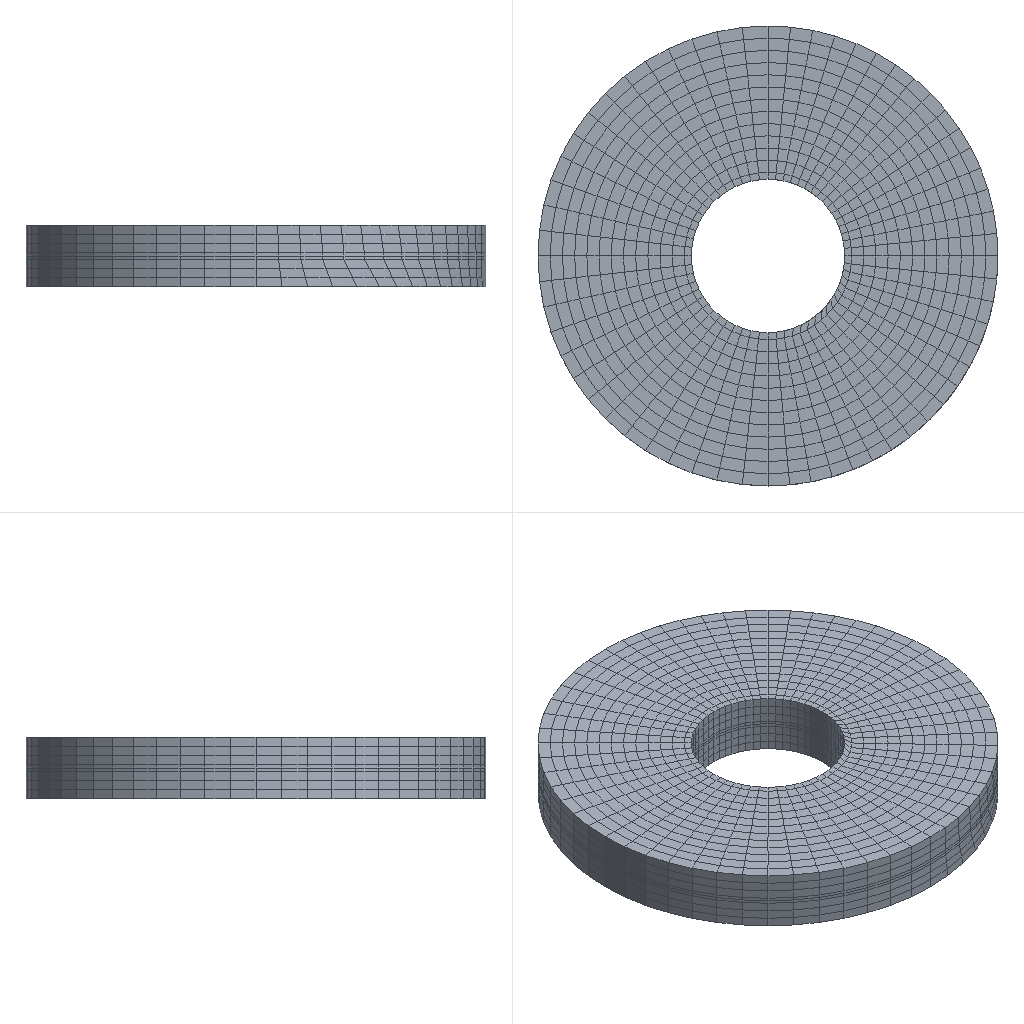Simulation study | abaqus
Set-up summary:
category,name,step,type,value,unit,region
solver,abaqus
solver,version,,,Abaqus/Explicit 2020
units,not stated in the deck,,not stated
analysis,deck,,transient,transient
load_step,Step-1,Step-1,transient
load_step,requested,,,1
mesh,nodes,,,8840
mesh,elements,,,7524
element_type,C3D8,,solid,6240
element_type,R3D3,,rigid,14
element_type,R3D4,,rigid,1270
load,load commands in deck,,count,1
bc,support commands in deck,,count,1
material,MATERIAL-1,,in results
material,MATERIAL-1-COPY,,in results
check,setup vs results,,match,"per instance, exact: element labels, types and connectivity; labels of the nodes the elements use; coordinates not compared"
Abaqus input file, long lists of numbers shortened:
*Heading
** Job name: Job-3 Model name: Model-1-Copy-Copy
** Generated by: Abaqus/CAE 2020
*Preprint, echo=NO, model=NO, history=NO, contact=NO
**
** PARTS
**
*Part, name=Part-1
*Node
      1,   1.118,  -2.236,           4.
      2,   1.118,  -2.236,           0.
** (1277 more lines like these left out)
*Element, type=R3D4
  1,   1,   3, 105, 156
  2,   3,   4, 106, 105
** (1268 more lines like these left out)
*Element, type=R3D3
677,  963,  757,  736
678,  987,  863,  818
** (12 more lines like these left out)
*Node
   1280,           0., -1.5308085e-16,           4.
*Nset, nset=Part-1-RefPt_, internal
1280,
*Elset, elset=Part-1, generate
    1,  1284,     1
*End Part
**
*Part, name=Part-2
*Node
      1,           0.,   2.723,  0.9
      2,           0.,          7.5,  0.9
** (7558 more lines like these left out)
*Element, type=C3D8
  1,    5,  117, 1334,  168,    1,   65, 1169,  116
  2,  117,  118, 1335, 1334,   65,   66, 1170, 1169
** (6238 more lines like these left out)
*Nset, nset=Set-3, generate
    1,  7560,     1
*Elset, elset=Set-3, generate
    1,  6240,     1
*Nset, nset=Set-11
    1,    2,    3,    4,    5,    6,    7,    8,    9,   10,   11,   12,   13,   14,   15,   16
   25,   26,   27,   28,   29,   30,   31,   32,   33,   39,   40,   41,   42,   43,   44,   47
** (437 more lines like these left out)
*Elset, elset=Set-11
    1,    2,    3,    4,    5,    6,    7,    8,    9,   10,   11,   12,   13,   14,   15,   16
   17,   18,   19,   20,   21,   22,   23,   24,   25,   26,   27,   28,   29,   30,   31,   32
** (358 more lines like these left out)
*Nset, nset=Set-12, generate
    1,  7560,     1
*Elset, elset=Set-12, generate
    1,  6240,     1
*Nset, nset=Set-9
    1,    2,    3,    4,    5,    6,    7,    8,    9,   10,   11,   12,   13,   14,   15,   16
   17,   18,   21,   22,   25,   26,   27,   28,   29,   30,   31,   32,   33,   34,   35,   36
** (467 more lines like these left out)
*Elset, elset=Set-9
    1,    2,    3,    4,    5,    6,    7,    8,    9,   10,   11,   12,   13,   14,   15,   16
   17,   18,   19,   20,   21,   22,   23,   24,   25,   26,   27,   28,   29,   30,   31,   32
** (381 more lines like these left out)
*Nset, nset=Set-10
    1,    4,    5,    8,    9,   11,   13,   15,   17,   18,   19,   20,   21,   22,   23,   24
   39,   42,   43,   45,   46,   47,   49,   50,  102,  103,  104,  105,  106,  107,  108,  109
** (21 more lines like these left out)
*Elset, elset=Set-10
  721,  722,  723,  724,  725,  726,  727,  728,  729,  730,  731,  732,  733,  734,  735,  736
  737,  738,  739,  740,  741,  742,  743,  744,  745,  746,  747,  748,  749,  750,  751,  752
** (6 more lines like these left out)
*Elset, elset=__PickedSurf25_S2, internal, generate
 6209,  6224,     1
*Elset, elset=__PickedSurf25_S1, internal
 3441, 3442, 3443, 3444, 3445, 3446, 3447, 3448, 3449, 3450, 3451, 3452, 3453, 3454, 3839, 3840
 3841, 3842, 3843, 3844, 3845, 3846, 3847, 3848, 3849, 3850, 3851, 3852, 3853, 3854, 3855, 3856
** (1 more lines like these left out)
*Surface, type=ELEMENT, name=_PickedSurf25, internal
__PickedSurf25_S2, S2
__PickedSurf25_S1, S1
** Section: Section-1
*Solid Section, elset=Set-9, material=Material-1
,
** Section: Section-3
*Solid Section, elset=Set-10, material=Material-1-Copy
,
*End Part
**
**
** ASSEMBLY
**
*Assembly, name=Assembly
**
*Instance, name=Part-1-1, part=Part-1
*End Instance
**
*Instance, name=Part-2-1, part=Part-2
          0.,           0.,           1.
*End Instance
**
*Nset, nset=Set-1, instance=Part-1-1
    1,    2,    3,    4,    5,    6,    7,    8,    9,   10,   11,   12,   13,   14,   15,   16
   17,   18,   19,   20,   21,   22,   23,   24,   25,   26,   27,   28,   29,   30,   31,   32
** (39 more lines like these left out)
*Elset, elset=Set-1, instance=Part-1-1, generate
  677,  1284,     1
*Nset, nset=Set-2, instance=Part-1-1
 1280,
*Elset, elset=_Surf-9_S4, internal, instance=Part-2-1
   12,   24,   36,   48,   60,   72,   84,   96,  108,  120,  132,  144,  156,  168,  180,  192
  396,  408,  420,  432,  444,  456,  468,  480,  492,  504,  516,  528,  540,  552,  564,  576
** (12 more lines like these left out)
*Elset, elset=_Surf-9_S5, internal, instance=Part-2-1
  369,  370,  371,  372,  373,  374,  375,  376,  377,  378,  379,  380,  381,  382,  383,  384
 1517, 1518, 1519, 1520, 1521, 1522, 1523, 1524, 1525, 1526, 1527, 1528, 1529, 1530, 1531, 1532
** (12 more lines like these left out)
*Elset, elset=_Surf-9_S3, internal, instance=Part-2-1
 3869, 3870, 3871, 3872, 3873, 3874, 3875, 3876, 3877, 3878, 3879, 3880, 3881, 3882, 4037, 4038
 4039, 4040, 4041, 4042, 4043, 4044, 4045, 4046, 4047, 4048, 4049, 4050, 4205, 4206, 4207, 4208
** (1 more lines like these left out)
*Surface, type=ELEMENT, name=Surf-9
_Surf-9_S4, S4
_Surf-9_S5, S5
_Surf-9_S3, S3
*Elset, elset=_m_Surf-1_SPOS, internal, instance=Part-1-1, generate
   1,  676,    1
*Surface, type=ELEMENT, name=m_Surf-1
_m_Surf-1_SPOS, SPOS
*Elset, elset=_m_Surf-4_SPOS, internal, instance=Part-1-1, generate
   1,  676,    1
*Surface, type=ELEMENT, name=m_Surf-4
_m_Surf-4_SPOS, SPOS
*Rigid Body, ref node=Part-1-1.Part-1-RefPt_, elset=Part-1-1.Part-1
*End Assembly
*Amplitude, name=Amp-1
             0.,              0.,              1.,              1.
**
** MATERIALS
**
*Material, name=Material-1
*Density
 1e-09,
*Elastic
75800., 0.24
*Material, name=Material-1-Copy
*Brittle Cracking
20.,    0.
16., 7e-06
*Brittle Shear
1.,    0.
0., 1e-05
*Brittle Failure
 1e-05,
*Density
 1e-09,
*Elastic
75800., 0.24
**
** INTERACTION PROPERTIES
**
*Surface Interaction, name=IntProp-1
*Friction
 0.2,
*Surface Behavior, pressure-overclosure=HARD
*Surface Interaction, name=IntProp-2
** ----------------------------------------------------------------
**
** STEP: Step-1
**
*Step, name=Step-1, nlgeom=YES
*Dynamic, Explicit
, 0.01
*Bulk Viscosity
0.06, 1.2
** Mass Scaling: Semi-Automatic
**               Whole Model
*Fixed Mass Scaling, factor=500.
**
** BOUNDARY CONDITIONS
**
** Name: BC-1 Type: 对称/反对称/完全固定
*Boundary
Set-2, ENCASTRE
**
** LOADS
**
** Name: Load-1   Type: Pressure
*Dsload
Surf-9, P, 50.
**
** OUTPUT REQUESTS
**
*Restart, write, number interval=1, time marks=NO
**
** FIELD OUTPUT: F-Output-1
**
*Output, field
*Node Output
CF, RF, U, V
*Element Output, directions=YES
DMICRT, E, LE, MISES, MISESMAX, PE, PEEQ, PEMAG, S, SDEG, STATUS
*Contact Output
CSDMG,
**
** HISTORY OUTPUT: H-Output-1
**
*Output, history, variable=PRESELECT, frequency=1
*End Step
Results summary:
result,step,Step-1,completed,increments=38834 time=0.01/0.01
result,analysis,,,transient
result,last_loadstep,,,1
result,primary field,,,U
result,reaction total,,FX,0.0,model units
result,reaction total,,FY,0.0,model units
result,reaction total,,FZ,0.0,model units